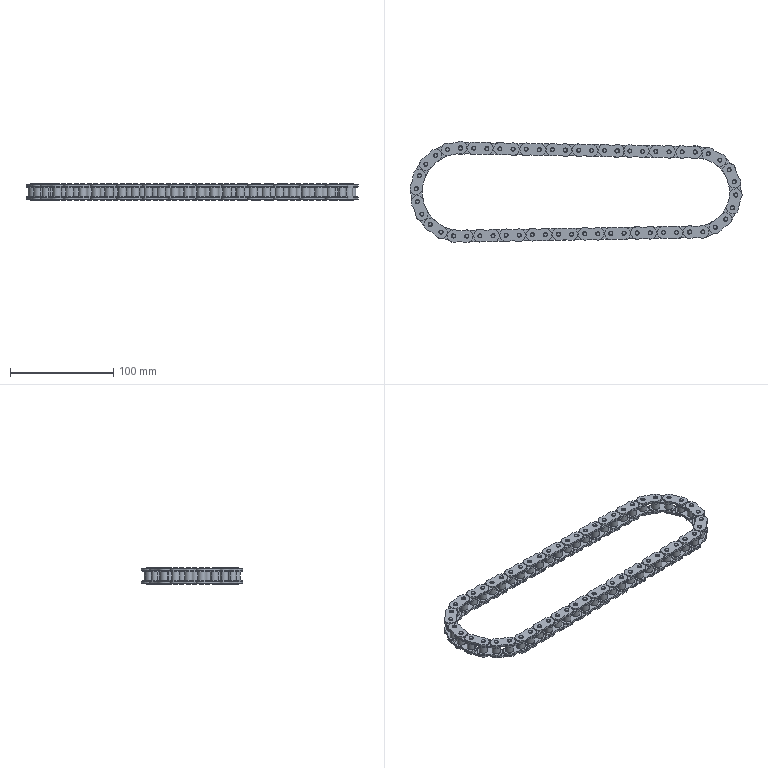Part | STEP file | Motor chain 1 | 84 solids | 1680 faces | box 321.643 x 97.927 x 16.175 mm | volume 70929 mm3 | cylinder 1120 | plane 336 | cone 224 | commonest cylinder face diameters 3.98 x448 12.07 x336 55.348 x224 7.92 x112